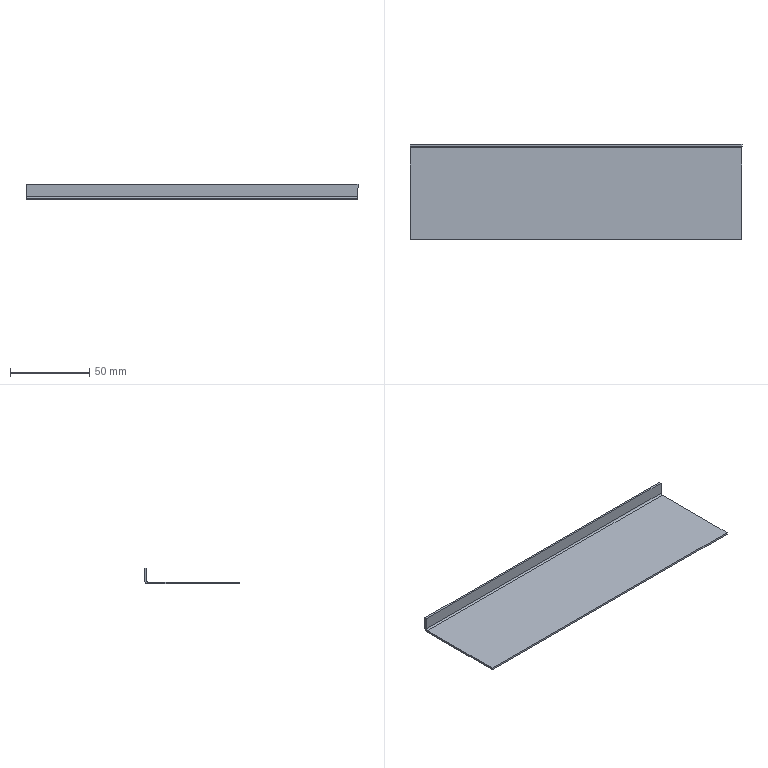Part | SolidWorks | features EdgeFlange 1, FlatPattern 1, HoleWzd 1, SMBaseFlange 1, SheetMetal 1 | 1 solid | 14 faces | box 209 x 60 x 10 mm | volume 17083 mm3 | plane 12 | cylinder 2 | commonest cylinder face diameters 2 x1 4.4 x1
STEP:
#1=CARTESIAN_POINT('',(-104.5,27.8,0.));
#2=VERTEX_POINT('',#1);
#3=CARTESIAN_POINT('',(-104.5,-30.,0.));
#4=VERTEX_POINT('',#3);
#5=CARTESIAN_POINT('',(-104.5,30.,0.));
#6=DIRECTION('',(0.,-1.,0.));
#7=VECTOR('',#6,1000.);
#8=LINE('',#5,#7);
#9=EDGE_CURVE('',#2,#4,#8,.T.);
#10=ORIENTED_EDGE('',*,*,#9,.F.);
#11=CARTESIAN_POINT('',(-104.5,27.8,-1.2));
#12=VERTEX_POINT('',#11);
#13=CARTESIAN_POINT('',(-104.5,27.8,0.));
#14=DIRECTION('',(0.,0.,-1.));
#15=VECTOR('',#14,1000.);
#16=LINE('',#13,#15);
#17=EDGE_CURVE('',#2,#12,#16,.T.);
#18=ORIENTED_EDGE('',*,*,#17,.T.);
#19=CARTESIAN_POINT('',(-104.5,-30.,-1.2));
#20=VERTEX_POINT('',#19);
#21=CARTESIAN_POINT('',(-104.5,30.,-1.2));
#22=DIRECTION('',(0.,-1.,0.));
#23=VECTOR('',#22,1000.);
#24=LINE('',#21,#23);
#25=EDGE_CURVE('',#12,#20,#24,.T.);
#26=ORIENTED_EDGE('',*,*,#25,.T.);
#27=CARTESIAN_POINT('',(-104.5,-30.,-1.2));
#28=DIRECTION('',(0.,0.,1.));
#29=VECTOR('',#28,1000.);
#30=LINE('',#27,#29);
#31=EDGE_CURVE('',#20,#4,#30,.T.);
#32=ORIENTED_EDGE('',*,*,#31,.T.);
#33=EDGE_LOOP('',(#10,#18,#26,#32));
#34=FACE_OUTER_BOUND('',#33,.T.);
#35=CARTESIAN_POINT('',(-104.5,30.,-1.2));
#36=DIRECTION('',(-1.,0.,0.));
#37=DIRECTION('',(0.,-1.,0.));
#38=AXIS2_PLACEMENT_3D('',#35,#36,#37);
#39=PLANE('',#38);
#40=ADVANCED_FACE('',(#34),#39,.T.);
#41=CARTESIAN_POINT('',(104.5,27.8,-1.2));
#42=VERTEX_POINT('',#41);
#43=CARTESIAN_POINT('',(-104.5,27.8,-1.2));
#44=DIRECTION('',(1.,0.,0.));
#45=VECTOR('',#44,1000.);
#46=LINE('',#43,#45);
#47=EDGE_CURVE('',#12,#42,#46,.T.);
#48=ORIENTED_EDGE('',*,*,#47,.T.);
#49=CARTESIAN_POINT('',(104.5,-30.,-1.2));
#50=VERTEX_POINT('',#49);
#51=CARTESIAN_POINT('',(104.5,30.,-1.2));
#52=DIRECTION('',(0.,1.,0.));
#53=VECTOR('',#52,1000.);
#54=LINE('',#51,#53);
#55=EDGE_CURVE('',#50,#42,#54,.T.);
#56=ORIENTED_EDGE('',*,*,#55,.F.);
#57=CARTESIAN_POINT('',(-104.5,-30.,-1.2));
#58=DIRECTION('',(1.,0.,0.));
#59=VECTOR('',#58,1000.);
#60=LINE('',#57,#59);
#61=EDGE_CURVE('',#20,#50,#60,.T.);
#62=ORIENTED_EDGE('',*,*,#61,.F.);
#63=ORIENTED_EDGE('',*,*,#25,.F.);
#64=EDGE_LOOP('',(#48,#56,#62,#63));
#65=FACE_OUTER_BOUND('',#64,.T.);
#66=CARTESIAN_POINT('',(0.,0.,-1.2));
#67=DIRECTION('',(0.,0.,1.));
#68=DIRECTION('',(1.,0.,0.));
#69=AXIS2_PLACEMENT_3D('',#66,#67,#68);
#70=PLANE('',#69);
#71=ADVANCED_FACE('',(#65),#70,.F.);
#72=CARTESIAN_POINT('',(104.5,-30.,0.));
#73=VERTEX_POINT('',#72);
#74=CARTESIAN_POINT('',(104.5,27.8,0.));
#75=VERTEX_POINT('',#74);
#76=CARTESIAN_POINT('',(104.5,30.,0.));
#77=DIRECTION('',(0.,1.,0.));
#78=VECTOR('',#77,1000.);
#79=LINE('',#76,#78);
#80=EDGE_CURVE('',#73,#75,#79,.T.);
#81=ORIENTED_EDGE('',*,*,#80,.T.);
#82=CARTESIAN_POINT('',(-104.5,27.8,0.));
#83=DIRECTION('',(1.,0.,0.));
#84=VECTOR('',#83,1000.);
#85=LINE('',#82,#84);
#86=EDGE_CURVE('',#2,#75,#85,.T.);
#87=ORIENTED_EDGE('',*,*,#86,.F.);
#88=ORIENTED_EDGE('',*,*,#9,.T.);
#89=CARTESIAN_POINT('',(-104.5,-30.,0.));
#90=DIRECTION('',(1.,0.,0.));
#91=VECTOR('',#90,1000.);
#92=LINE('',#89,#91);
#93=EDGE_CURVE('',#4,#73,#92,.T.);
#94=ORIENTED_EDGE('',*,*,#93,.T.);
#95=EDGE_LOOP('',(#81,#87,#88,#94));
#96=FACE_OUTER_BOUND('',#95,.T.);
#97=CARTESIAN_POINT('',(0.,0.,0.));
#98=DIRECTION('',(0.,0.,1.));
#99=DIRECTION('',(1.,0.,0.));
#100=AXIS2_PLACEMENT_3D('',#97,#98,#99);
#101=PLANE('',#100);
#102=ADVANCED_FACE('',(#96),#101,.T.);
#103=CARTESIAN_POINT('',(104.5,27.8,0.));
#104=DIRECTION('',(0.,0.,-1.));
#105=VECTOR('',#104,1000.);
#106=LINE('',#103,#105);
#107=EDGE_CURVE('',#75,#42,#106,.T.);
#108=ORIENTED_EDGE('',*,*,#107,.F.);
#109=ORIENTED_EDGE('',*,*,#80,.F.);
#110=CARTESIAN_POINT('',(104.5,-30.,-1.2));
#111=DIRECTION('',(0.,0.,1.));
#112=VECTOR('',#111,1000.);
#113=LINE('',#110,#112);
#114=EDGE_CURVE('',#50,#73,#113,.T.);
#115=ORIENTED_EDGE('',*,*,#114,.F.);
#116=ORIENTED_EDGE('',*,*,#55,.T.);
#117=EDGE_LOOP('',(#108,#109,#115,#116));
#118=FACE_OUTER_BOUND('',#117,.T.);
#119=CARTESIAN_POINT('',(104.5,30.,-1.2));
#120=DIRECTION('',(1.,0.,0.));
#121=DIRECTION('',(0.,1.,0.));
#122=AXIS2_PLACEMENT_3D('',#119,#120,#121);
#123=PLANE('',#122);
#124=ADVANCED_FACE('',(#118),#123,.T.);
#125=ORIENTED_EDGE('',*,*,#93,.F.);
#126=ORIENTED_EDGE('',*,*,#31,.F.);
#127=ORIENTED_EDGE('',*,*,#61,.T.);
#128=ORIENTED_EDGE('',*,*,#114,.T.);
#129=EDGE_LOOP('',(#125,#126,#127,#128));
#130=FACE_OUTER_BOUND('',#129,.T.);
#131=CARTESIAN_POINT('',(-104.5,-30.,-1.2));
#132=DIRECTION('',(0.,-1.,0.));
#133=DIRECTION('',(0.,0.,-1.));
#134=AXIS2_PLACEMENT_3D('',#131,#132,#133);
#135=PLANE('',#134);
#136=ADVANCED_FACE('',(#130),#135,.T.);
#137=CARTESIAN_POINT('',(104.5,28.8,1.));
#138=VERTEX_POINT('',#137);
#139=CARTESIAN_POINT('',(104.5,30.,1.));
#140=VERTEX_POINT('',#139);
#141=CARTESIAN_POINT('',(104.5,30.,1.));
#142=DIRECTION('',(0.,1.,0.));
#143=VECTOR('',#142,1000.);
#144=LINE('',#141,#143);
#145=EDGE_CURVE('',#138,#140,#144,.T.);
#146=ORIENTED_EDGE('',*,*,#145,.F.);
#147=CARTESIAN_POINT('',(104.5,27.8,1.));
#148=DIRECTION('',(1.,0.,0.));
#149=DIRECTION('',(0.,0.,1.));
#150=AXIS2_PLACEMENT_3D('',#147,#148,#149);
#151=CIRCLE('',#150,1.);
#152=EDGE_CURVE('',#75,#138,#151,.T.);
#153=ORIENTED_EDGE('',*,*,#152,.F.);
#154=ORIENTED_EDGE('',*,*,#107,.T.);
#155=CARTESIAN_POINT('',(104.5,27.8,1.));
#156=DIRECTION('',(1.,0.,0.));
#157=DIRECTION('',(0.,0.,1.));
#158=AXIS2_PLACEMENT_3D('',#155,#156,#157);
#159=CIRCLE('',#158,2.2);
#160=EDGE_CURVE('',#42,#140,#159,.T.);
#161=ORIENTED_EDGE('',*,*,#160,.T.);
#162=EDGE_LOOP('',(#146,#153,#154,#161));
#163=FACE_OUTER_BOUND('',#162,.T.);
#164=CARTESIAN_POINT('',(104.5,27.8,1.));
#165=DIRECTION('',(1.,0.,0.));
#166=DIRECTION('',(0.,0.,-1.));
#167=AXIS2_PLACEMENT_3D('',#164,#165,#166);
#168=PLANE('',#167);
#169=ADVANCED_FACE('',(#163),#168,.T.);
#170=CARTESIAN_POINT('',(-104.5,28.8,1.));
#171=VERTEX_POINT('',#170);
#172=CARTESIAN_POINT('',(-104.5,27.8,1.));
#173=DIRECTION('',(-1.,0.,0.));
#174=DIRECTION('',(0.,0.,1.));
#175=AXIS2_PLACEMENT_3D('',#172,#173,#174);
#176=CIRCLE('',#175,1.);
#177=EDGE_CURVE('',#171,#2,#176,.T.);
#178=ORIENTED_EDGE('',*,*,#177,.F.);
#179=CARTESIAN_POINT('',(-104.5,30.,1.));
#180=VERTEX_POINT('',#179);
#181=CARTESIAN_POINT('',(-104.5,28.8,1.));
#182=DIRECTION('',(0.,1.,0.));
#183=VECTOR('',#182,1000.);
#184=LINE('',#181,#183);
#185=EDGE_CURVE('',#171,#180,#184,.T.);
#186=ORIENTED_EDGE('',*,*,#185,.T.);
#187=CARTESIAN_POINT('',(-104.5,27.8,1.));
#188=DIRECTION('',(-1.,0.,0.));
#189=DIRECTION('',(0.,0.,1.));
#190=AXIS2_PLACEMENT_3D('',#187,#188,#189);
#191=CIRCLE('',#190,2.2);
#192=EDGE_CURVE('',#180,#12,#191,.T.);
#193=ORIENTED_EDGE('',*,*,#192,.T.);
#194=ORIENTED_EDGE('',*,*,#17,.F.);
#195=EDGE_LOOP('',(#178,#186,#193,#194));
#196=FACE_OUTER_BOUND('',#195,.T.);
#197=CARTESIAN_POINT('',(-104.5,27.8,1.));
#198=DIRECTION('',(1.,0.,0.));
#199=DIRECTION('',(0.,0.,-1.));
#200=AXIS2_PLACEMENT_3D('',#197,#198,#199);
#201=PLANE('',#200);
#202=ADVANCED_FACE('',(#196),#201,.F.);
#203=ORIENTED_EDGE('',*,*,#47,.F.);
#204=ORIENTED_EDGE('',*,*,#192,.F.);
#205=CARTESIAN_POINT('',(104.5,30.,1.));
#206=DIRECTION('',(1.,0.,0.));
#207=VECTOR('',#206,1000.);
#208=LINE('',#205,#207);
#209=EDGE_CURVE('',#180,#140,#208,.T.);
#210=ORIENTED_EDGE('',*,*,#209,.T.);
#211=ORIENTED_EDGE('',*,*,#160,.F.);
#212=EDGE_LOOP('',(#203,#204,#210,#211));
#213=FACE_OUTER_BOUND('',#212,.T.);
#214=CARTESIAN_POINT('',(-104.5,27.8,1.));
#215=DIRECTION('',(-1.,0.,0.));
#216=DIRECTION('',(0.,1.,0.));
#217=AXIS2_PLACEMENT_3D('',#214,#215,#216);
#218=CYLINDRICAL_SURFACE('',#217,2.2);
#219=ADVANCED_FACE('',(#213),#218,.T.);
#220=ORIENTED_EDGE('',*,*,#86,.T.);
#221=ORIENTED_EDGE('',*,*,#152,.T.);
#222=CARTESIAN_POINT('',(104.5,28.8,1.));
#223=DIRECTION('',(-1.,0.,0.));
#224=VECTOR('',#223,1000.);
#225=LINE('',#222,#224);
#226=EDGE_CURVE('',#138,#171,#225,.T.);
#227=ORIENTED_EDGE('',*,*,#226,.T.);
#228=ORIENTED_EDGE('',*,*,#177,.T.);
#229=EDGE_LOOP('',(#220,#221,#227,#228));
#230=FACE_OUTER_BOUND('',#229,.T.);
#231=CARTESIAN_POINT('',(-104.5,27.8,1.));
#232=DIRECTION('',(-1.,0.,0.));
#233=DIRECTION('',(0.,1.,0.));
#234=AXIS2_PLACEMENT_3D('',#231,#232,#233);
#235=CYLINDRICAL_SURFACE('',#234,1.);
#236=ADVANCED_FACE('',(#230),#235,.F.);
#237=ORIENTED_EDGE('',*,*,#145,.T.);
#238=CARTESIAN_POINT('',(104.5,30.,8.8));
#239=VERTEX_POINT('',#238);
#240=CARTESIAN_POINT('',(104.5,30.,0.));
#241=DIRECTION('',(0.,0.,-1.));
#242=VECTOR('',#241,1000.);
#243=LINE('',#240,#242);
#244=EDGE_CURVE('',#239,#140,#243,.T.);
#245=ORIENTED_EDGE('',*,*,#244,.F.);
#246=CARTESIAN_POINT('',(104.5,28.8,8.8));
#247=VERTEX_POINT('',#246);
#248=CARTESIAN_POINT('',(104.5,30.,8.8));
#249=DIRECTION('',(0.,-1.,0.));
#250=VECTOR('',#249,1000.);
#251=LINE('',#248,#250);
#252=EDGE_CURVE('',#239,#247,#251,.T.);
#253=ORIENTED_EDGE('',*,*,#252,.T.);
#254=CARTESIAN_POINT('',(104.5,28.8,0.));
#255=DIRECTION('',(0.,0.,-1.));
#256=VECTOR('',#255,1000.);
#257=LINE('',#254,#256);
#258=EDGE_CURVE('',#247,#138,#257,.T.);
#259=ORIENTED_EDGE('',*,*,#258,.T.);
#260=EDGE_LOOP('',(#237,#245,#253,#259));
#261=FACE_OUTER_BOUND('',#260,.T.);
#262=CARTESIAN_POINT('',(104.5,30.,0.));
#263=DIRECTION('',(-1.,0.,0.));
#264=DIRECTION('',(0.,0.,1.));
#265=AXIS2_PLACEMENT_3D('',#262,#263,#264);
#266=PLANE('',#265);
#267=ADVANCED_FACE('',(#261),#266,.F.);
#268=ORIENTED_EDGE('',*,*,#185,.F.);
#269=CARTESIAN_POINT('',(-104.5,28.8,8.8));
#270=VERTEX_POINT('',#269);
#271=CARTESIAN_POINT('',(-104.5,28.8,8.8));
#272=DIRECTION('',(0.,0.,1.));
#273=VECTOR('',#272,1000.);
#274=LINE('',#271,#273);
#275=EDGE_CURVE('',#171,#270,#274,.T.);
#276=ORIENTED_EDGE('',*,*,#275,.T.);
#277=CARTESIAN_POINT('',(-104.5,30.,8.8));
#278=VERTEX_POINT('',#277);
#279=CARTESIAN_POINT('',(-104.5,30.,8.8));
#280=DIRECTION('',(0.,-1.,0.));
#281=VECTOR('',#280,1000.);
#282=LINE('',#279,#281);
#283=EDGE_CURVE('',#278,#270,#282,.T.);
#284=ORIENTED_EDGE('',*,*,#283,.F.);
#285=CARTESIAN_POINT('',(-104.5,30.,0.));
#286=DIRECTION('',(0.,0.,1.));
#287=VECTOR('',#286,1000.);
#288=LINE('',#285,#287);
#289=EDGE_CURVE('',#180,#278,#288,.T.);
#290=ORIENTED_EDGE('',*,*,#289,.F.);
#291=EDGE_LOOP('',(#268,#276,#284,#290));
#292=FACE_OUTER_BOUND('',#291,.T.);
#293=CARTESIAN_POINT('',(-104.5,30.,8.8));
#294=DIRECTION('',(1.,0.,0.));
#295=DIRECTION('',(0.,0.,-1.));
#296=AXIS2_PLACEMENT_3D('',#293,#294,#295);
#297=PLANE('',#296);
#298=ADVANCED_FACE('',(#292),#297,.F.);
#299=ORIENTED_EDGE('',*,*,#209,.F.);
#300=ORIENTED_EDGE('',*,*,#289,.T.);
#301=CARTESIAN_POINT('',(0.,30.,8.8));
#302=DIRECTION('',(1.,0.,0.));
#303=VECTOR('',#302,1000.);
#304=LINE('',#301,#303);
#305=EDGE_CURVE('',#278,#239,#304,.T.);
#306=ORIENTED_EDGE('',*,*,#305,.T.);
#307=ORIENTED_EDGE('',*,*,#244,.T.);
#308=EDGE_LOOP('',(#299,#300,#306,#307));
#309=FACE_OUTER_BOUND('',#308,.T.);
#310=CARTESIAN_POINT('',(0.,30.,0.));
#311=DIRECTION('',(0.,-1.,0.));
#312=DIRECTION('',(0.,0.,-1.));
#313=AXIS2_PLACEMENT_3D('',#310,#311,#312);
#314=PLANE('',#313);
#315=ADVANCED_FACE('',(#309),#314,.F.);
#316=ORIENTED_EDGE('',*,*,#275,.F.);
#317=ORIENTED_EDGE('',*,*,#226,.F.);
#318=ORIENTED_EDGE('',*,*,#258,.F.);
#319=CARTESIAN_POINT('',(104.5,28.8,8.8));
#320=DIRECTION('',(1.,0.,0.));
#321=VECTOR('',#320,1000.);
#322=LINE('',#319,#321);
#323=EDGE_CURVE('',#270,#247,#322,.T.);
#324=ORIENTED_EDGE('',*,*,#323,.F.);
#325=EDGE_LOOP('',(#316,#317,#318,#324));
#326=FACE_OUTER_BOUND('',#325,.T.);
#327=CARTESIAN_POINT('',(0.,28.8,0.));
#328=DIRECTION('',(0.,-1.,0.));
#329=DIRECTION('',(0.,0.,-1.));
#330=AXIS2_PLACEMENT_3D('',#327,#328,#329);
#331=PLANE('',#330);
#332=ADVANCED_FACE('',(#326),#331,.T.);
#333=ORIENTED_EDGE('',*,*,#323,.T.);
#334=ORIENTED_EDGE('',*,*,#252,.F.);
#335=ORIENTED_EDGE('',*,*,#305,.F.);
#336=ORIENTED_EDGE('',*,*,#283,.T.);
#337=EDGE_LOOP('',(#333,#334,#335,#336));
#338=FACE_OUTER_BOUND('',#337,.T.);
#339=CARTESIAN_POINT('',(104.5,30.,8.8));
#340=DIRECTION('',(0.,0.,-1.));
#341=DIRECTION('',(0.,1.,0.));
#342=AXIS2_PLACEMENT_3D('',#339,#340,#341);
#343=PLANE('',#342);
#344=ADVANCED_FACE('',(#338),#343,.F.);
#345=CLOSED_SHELL('',(#40,#71,#102,#124,#136,#169,#202,#219,#236,#267,#298,#315,#332,#344));
#346=MANIFOLD_SOLID_BREP('',#345);
#347=CARTESIAN_POINT('',(0.,0.,0.));
#348=DIRECTION('',(0.,0.,1.));
#349=DIRECTION('',(1.,0.,0.));
#350=AXIS2_PLACEMENT_3D('',#347,#348,#349);
#351=(LENGTH_UNIT()NAMED_UNIT(*)SI_UNIT(.MILLI.,.METRE.));
#352=UNCERTAINTY_MEASURE_WITH_UNIT(LENGTH_MEASURE(0.00001),#351,'','');
#353=(NAMED_UNIT(*)PLANE_ANGLE_UNIT()SI_UNIT($,.RADIAN.));
#354=(NAMED_UNIT(*)SI_UNIT($,.STERADIAN.)SOLID_ANGLE_UNIT());
#355=(GEOMETRIC_REPRESENTATION_CONTEXT(3)GLOBAL_UNCERTAINTY_ASSIGNED_CONTEXT((#352))GLOBAL_UNIT_ASSIGNED_CONTEXT((#351,#353,#354))REPRESENTATION_CONTEXT('',''));
#356=ADVANCED_BREP_SHAPE_REPRESENTATION('',(#346,#350),#355);